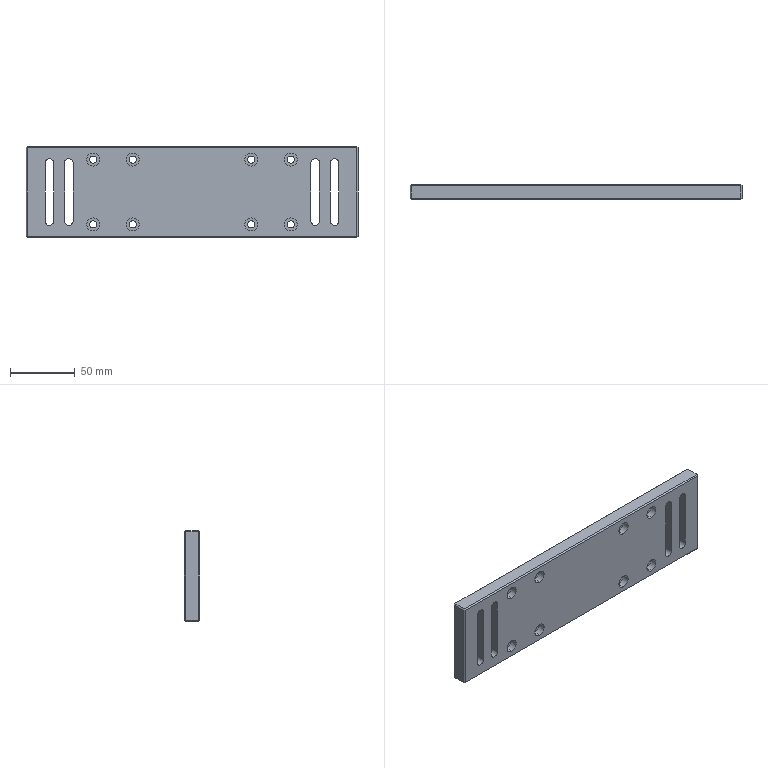Part | STEP file | BPSP-11-09 Pusher Fixing Plate_Default | 1 solid | 98 faces | box 256 x 12 x 70 mm | volume 193349 mm3 | cylinder 50 | plane 42 | cone 6 | commonest cylinder face diameters 5.5 x16 10 x16 6.5 x12 4.2 x6